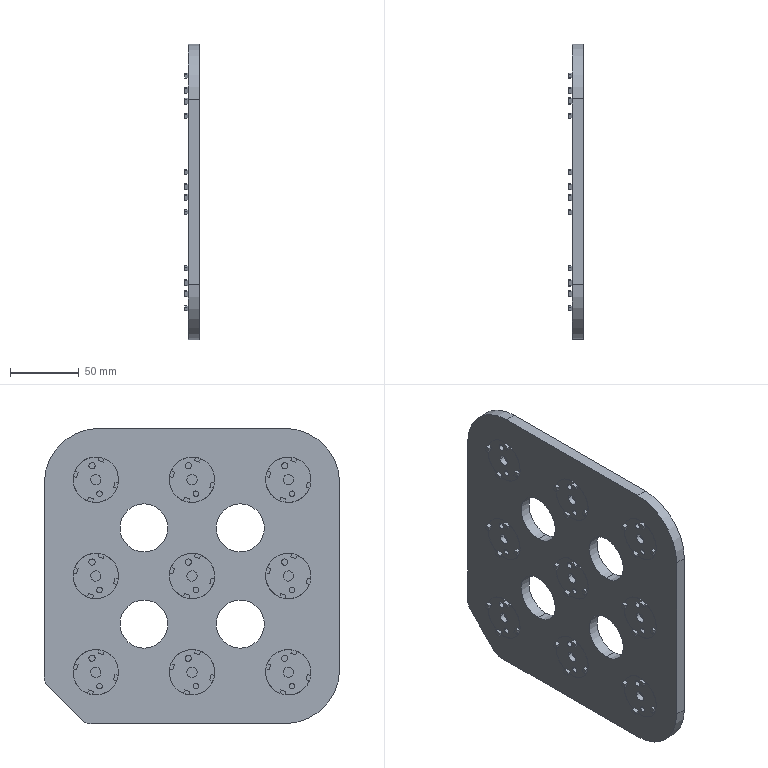Part | SolidWorks | features MoveCopyBody 6, ICE 5, Fillet 2, LPattern 2, MoveFace 2, Chamfer 1, Cut 1, Extrusion 1, Stock 1 | 1 solid | 272 faces | box 10.7 x 214.9 x 214.8 mm | volume 326451 mm3 | plane 187 | cylinder 85 | commonest cylinder face diameters 4 x18 4.5 x18 7.5 x18 33 x18 35 x8 80 x3